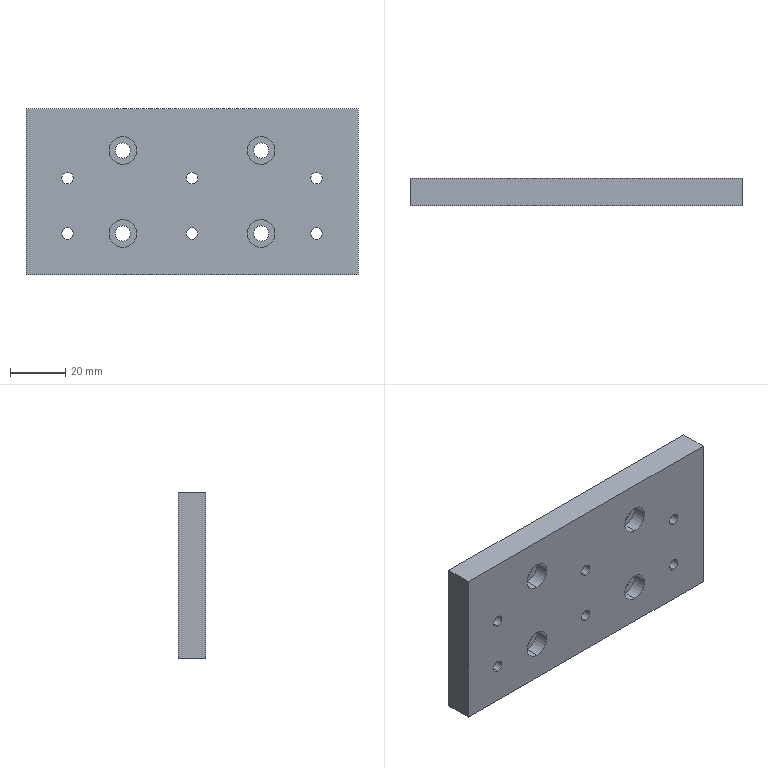Part | SolidWorks | features HoleWzd 2, LPattern 2, Extrusion 1 | 1 solid | 38 faces | box 120 x 10 x 60 mm | volume 69123 mm3 | cylinder 28 | plane 10 | commonest cylinder face diameters 4.2 x12 5.5 x8 10 x8
STEP:
#1=CARTESIAN_POINT('',(45.,10.,-12.9));
#2=VERTEX_POINT('',#1);
#3=CARTESIAN_POINT('',(45.,10.,-17.1));
#4=VERTEX_POINT('',#3);
#5=CARTESIAN_POINT('',(45.,10.,-15.));
#6=DIRECTION('',(0.,-1.,0.));
#7=DIRECTION('',(0.,0.,-1.));
#8=AXIS2_PLACEMENT_3D('',#5,#6,#7);
#9=CIRCLE('',#8,2.1);
#10=EDGE_CURVE('',#2,#4,#9,.T.);
#11=ORIENTED_EDGE('',*,*,#10,.F.);
#12=CARTESIAN_POINT('',(45.,0.,-12.9));
#13=VERTEX_POINT('',#12);
#14=CARTESIAN_POINT('',(45.,0.,-12.9));
#15=DIRECTION('',(0.,-1.,0.));
#16=VECTOR('',#15,1000.);
#17=LINE('',#14,#16);
#18=EDGE_CURVE('',#2,#13,#17,.T.);
#19=ORIENTED_EDGE('',*,*,#18,.T.);
#20=CARTESIAN_POINT('',(45.,0.,-17.1));
#21=VERTEX_POINT('',#20);
#22=CARTESIAN_POINT('',(45.,0.,-15.));
#23=DIRECTION('',(0.,-1.,0.));
#24=DIRECTION('',(0.,0.,-1.));
#25=AXIS2_PLACEMENT_3D('',#22,#23,#24);
#26=CIRCLE('',#25,2.1);
#27=EDGE_CURVE('',#13,#21,#26,.T.);
#28=ORIENTED_EDGE('',*,*,#27,.T.);
#29=CARTESIAN_POINT('',(45.,0.,-17.1));
#30=DIRECTION('',(0.,-1.,0.));
#31=VECTOR('',#30,1000.);
#32=LINE('',#29,#31);
#33=EDGE_CURVE('',#4,#21,#32,.T.);
#34=ORIENTED_EDGE('',*,*,#33,.F.);
#35=EDGE_LOOP('',(#11,#19,#28,#34));
#36=FACE_OUTER_BOUND('',#35,.T.);
#37=CARTESIAN_POINT('',(45.,0.,-15.));
#38=DIRECTION('',(0.,-1.,0.));
#39=DIRECTION('',(0.,0.,-1.));
#40=AXIS2_PLACEMENT_3D('',#37,#38,#39);
#41=CYLINDRICAL_SURFACE('',#40,2.1);
#42=ADVANCED_FACE('',(#36),#41,.F.);
#43=CARTESIAN_POINT('',(0.,10.,-12.9));
#44=VERTEX_POINT('',#43);
#45=CARTESIAN_POINT('',(0.,10.,-17.1));
#46=VERTEX_POINT('',#45);
#47=CARTESIAN_POINT('',(0.,10.,-15.));
#48=DIRECTION('',(0.,-1.,0.));
#49=DIRECTION('',(0.,0.,-1.));
#50=AXIS2_PLACEMENT_3D('',#47,#48,#49);
#51=CIRCLE('',#50,2.1);
#52=EDGE_CURVE('',#44,#46,#51,.T.);
#53=ORIENTED_EDGE('',*,*,#52,.F.);
#54=CARTESIAN_POINT('',(0.,0.,-12.9));
#55=VERTEX_POINT('',#54);
#56=CARTESIAN_POINT('',(0.,0.,-12.9));
#57=DIRECTION('',(0.,-1.,0.));
#58=VECTOR('',#57,1000.);
#59=LINE('',#56,#58);
#60=EDGE_CURVE('',#44,#55,#59,.T.);
#61=ORIENTED_EDGE('',*,*,#60,.T.);
#62=CARTESIAN_POINT('',(0.,0.,-17.1));
#63=VERTEX_POINT('',#62);
#64=CARTESIAN_POINT('',(0.,0.,-15.));
#65=DIRECTION('',(0.,-1.,0.));
#66=DIRECTION('',(0.,0.,-1.));
#67=AXIS2_PLACEMENT_3D('',#64,#65,#66);
#68=CIRCLE('',#67,2.1);
#69=EDGE_CURVE('',#55,#63,#68,.T.);
#70=ORIENTED_EDGE('',*,*,#69,.T.);
#71=CARTESIAN_POINT('',(0.,0.,-17.1));
#72=DIRECTION('',(0.,-1.,0.));
#73=VECTOR('',#72,1000.);
#74=LINE('',#71,#73);
#75=EDGE_CURVE('',#46,#63,#74,.T.);
#76=ORIENTED_EDGE('',*,*,#75,.F.);
#77=EDGE_LOOP('',(#53,#61,#70,#76));
#78=FACE_OUTER_BOUND('',#77,.T.);
#79=CARTESIAN_POINT('',(0.,0.,-15.));
#80=DIRECTION('',(0.,-1.,0.));
#81=DIRECTION('',(0.,0.,-1.));
#82=AXIS2_PLACEMENT_3D('',#79,#80,#81);
#83=CYLINDRICAL_SURFACE('',#82,2.1);
#84=ADVANCED_FACE('',(#78),#83,.F.);
#85=CARTESIAN_POINT('',(-45.,10.,-12.9));
#86=VERTEX_POINT('',#85);
#87=CARTESIAN_POINT('',(-45.,10.,-17.1));
#88=VERTEX_POINT('',#87);
#89=CARTESIAN_POINT('',(-45.,10.,-15.));
#90=DIRECTION('',(0.,-1.,0.));
#91=DIRECTION('',(0.,0.,-1.));
#92=AXIS2_PLACEMENT_3D('',#89,#90,#91);
#93=CIRCLE('',#92,2.1);
#94=EDGE_CURVE('',#86,#88,#93,.T.);
#95=ORIENTED_EDGE('',*,*,#94,.F.);
#96=CARTESIAN_POINT('',(-45.,0.,-12.9));
#97=VERTEX_POINT('',#96);
#98=CARTESIAN_POINT('',(-45.,0.,-12.9));
#99=DIRECTION('',(0.,-1.,0.));
#100=VECTOR('',#99,1000.);
#101=LINE('',#98,#100);
#102=EDGE_CURVE('',#86,#97,#101,.T.);
#103=ORIENTED_EDGE('',*,*,#102,.T.);
#104=CARTESIAN_POINT('',(-45.,0.,-17.1));
#105=VERTEX_POINT('',#104);
#106=CARTESIAN_POINT('',(-45.,0.,-15.));
#107=DIRECTION('',(0.,-1.,0.));
#108=DIRECTION('',(0.,0.,-1.));
#109=AXIS2_PLACEMENT_3D('',#106,#107,#108);
#110=CIRCLE('',#109,2.1);
#111=EDGE_CURVE('',#97,#105,#110,.T.);
#112=ORIENTED_EDGE('',*,*,#111,.T.);
#113=CARTESIAN_POINT('',(-45.,0.,-17.1));
#114=DIRECTION('',(0.,-1.,0.));
#115=VECTOR('',#114,1000.);
#116=LINE('',#113,#115);
#117=EDGE_CURVE('',#88,#105,#116,.T.);
#118=ORIENTED_EDGE('',*,*,#117,.F.);
#119=EDGE_LOOP('',(#95,#103,#112,#118));
#120=FACE_OUTER_BOUND('',#119,.T.);
#121=CARTESIAN_POINT('',(-45.,0.,-15.));
#122=DIRECTION('',(0.,-1.,0.));
#123=DIRECTION('',(0.,0.,-1.));
#124=AXIS2_PLACEMENT_3D('',#121,#122,#123);
#125=CYLINDRICAL_SURFACE('',#124,2.1);
#126=ADVANCED_FACE('',(#120),#125,.F.);
#127=CARTESIAN_POINT('',(45.,10.,7.1));
#128=VERTEX_POINT('',#127);
#129=CARTESIAN_POINT('',(45.,10.,2.9));
#130=VERTEX_POINT('',#129);
#131=CARTESIAN_POINT('',(45.,10.,5.));
#132=DIRECTION('',(0.,-1.,0.));
#133=DIRECTION('',(0.,0.,-1.));
#134=AXIS2_PLACEMENT_3D('',#131,#132,#133);
#135=CIRCLE('',#134,2.1);
#136=EDGE_CURVE('',#128,#130,#135,.T.);
#137=ORIENTED_EDGE('',*,*,#136,.F.);
#138=CARTESIAN_POINT('',(45.,0.,7.1));
#139=VERTEX_POINT('',#138);
#140=CARTESIAN_POINT('',(45.,0.,7.1));
#141=DIRECTION('',(0.,-1.,0.));
#142=VECTOR('',#141,1000.);
#143=LINE('',#140,#142);
#144=EDGE_CURVE('',#128,#139,#143,.T.);
#145=ORIENTED_EDGE('',*,*,#144,.T.);
#146=CARTESIAN_POINT('',(45.,0.,2.9));
#147=VERTEX_POINT('',#146);
#148=CARTESIAN_POINT('',(45.,0.,5.));
#149=DIRECTION('',(0.,-1.,0.));
#150=DIRECTION('',(0.,0.,-1.));
#151=AXIS2_PLACEMENT_3D('',#148,#149,#150);
#152=CIRCLE('',#151,2.1);
#153=EDGE_CURVE('',#139,#147,#152,.T.);
#154=ORIENTED_EDGE('',*,*,#153,.T.);
#155=CARTESIAN_POINT('',(45.,0.,2.9));
#156=DIRECTION('',(0.,-1.,0.));
#157=VECTOR('',#156,1000.);
#158=LINE('',#155,#157);
#159=EDGE_CURVE('',#130,#147,#158,.T.);
#160=ORIENTED_EDGE('',*,*,#159,.F.);
#161=EDGE_LOOP('',(#137,#145,#154,#160));
#162=FACE_OUTER_BOUND('',#161,.T.);
#163=CARTESIAN_POINT('',(45.,0.,5.));
#164=DIRECTION('',(0.,-1.,0.));
#165=DIRECTION('',(0.,0.,-1.));
#166=AXIS2_PLACEMENT_3D('',#163,#164,#165);
#167=CYLINDRICAL_SURFACE('',#166,2.1);
#168=ADVANCED_FACE('',(#162),#167,.F.);
#169=CARTESIAN_POINT('',(0.,10.,7.1));
#170=VERTEX_POINT('',#169);
#171=CARTESIAN_POINT('',(0.,10.,2.9));
#172=VERTEX_POINT('',#171);
#173=CARTESIAN_POINT('',(0.,10.,5.));
#174=DIRECTION('',(0.,-1.,0.));
#175=DIRECTION('',(0.,0.,-1.));
#176=AXIS2_PLACEMENT_3D('',#173,#174,#175);
#177=CIRCLE('',#176,2.1);
#178=EDGE_CURVE('',#170,#172,#177,.T.);
#179=ORIENTED_EDGE('',*,*,#178,.F.);
#180=CARTESIAN_POINT('',(0.,0.,7.1));
#181=VERTEX_POINT('',#180);
#182=CARTESIAN_POINT('',(0.,0.,7.1));
#183=DIRECTION('',(0.,-1.,0.));
#184=VECTOR('',#183,1000.);
#185=LINE('',#182,#184);
#186=EDGE_CURVE('',#170,#181,#185,.T.);
#187=ORIENTED_EDGE('',*,*,#186,.T.);
#188=CARTESIAN_POINT('',(0.,0.,2.9));
#189=VERTEX_POINT('',#188);
#190=CARTESIAN_POINT('',(0.,0.,5.));
#191=DIRECTION('',(0.,-1.,0.));
#192=DIRECTION('',(0.,0.,-1.));
#193=AXIS2_PLACEMENT_3D('',#190,#191,#192);
#194=CIRCLE('',#193,2.1);
#195=EDGE_CURVE('',#181,#189,#194,.T.);
#196=ORIENTED_EDGE('',*,*,#195,.T.);
#197=CARTESIAN_POINT('',(0.,0.,2.9));
#198=DIRECTION('',(0.,-1.,0.));
#199=VECTOR('',#198,1000.);
#200=LINE('',#197,#199);
#201=EDGE_CURVE('',#172,#189,#200,.T.);
#202=ORIENTED_EDGE('',*,*,#201,.F.);
#203=EDGE_LOOP('',(#179,#187,#196,#202));
#204=FACE_OUTER_BOUND('',#203,.T.);
#205=CARTESIAN_POINT('',(0.,0.,5.));
#206=DIRECTION('',(0.,-1.,0.));
#207=DIRECTION('',(0.,0.,-1.));
#208=AXIS2_PLACEMENT_3D('',#205,#206,#207);
#209=CYLINDRICAL_SURFACE('',#208,2.1);
#210=ADVANCED_FACE('',(#204),#209,.F.);
#211=CARTESIAN_POINT('',(-45.,10.,7.1));
#212=VERTEX_POINT('',#211);
#213=CARTESIAN_POINT('',(-45.,10.,2.9));
#214=VERTEX_POINT('',#213);
#215=CARTESIAN_POINT('',(-45.,10.,5.));
#216=DIRECTION('',(0.,-1.,0.));
#217=DIRECTION('',(0.,0.,-1.));
#218=AXIS2_PLACEMENT_3D('',#215,#216,#217);
#219=CIRCLE('',#218,2.1);
#220=EDGE_CURVE('',#212,#214,#219,.T.);
#221=ORIENTED_EDGE('',*,*,#220,.F.);
#222=CARTESIAN_POINT('',(-45.,0.,7.1));
#223=VERTEX_POINT('',#222);
#224=CARTESIAN_POINT('',(-45.,0.,7.1));
#225=DIRECTION('',(0.,-1.,0.));
#226=VECTOR('',#225,1000.);
#227=LINE('',#224,#226);
#228=EDGE_CURVE('',#212,#223,#227,.T.);
#229=ORIENTED_EDGE('',*,*,#228,.T.);
#230=CARTESIAN_POINT('',(-45.,0.,2.9));
#231=VERTEX_POINT('',#230);
#232=CARTESIAN_POINT('',(-45.,0.,5.));
#233=DIRECTION('',(0.,-1.,0.));
#234=DIRECTION('',(0.,0.,-1.));
#235=AXIS2_PLACEMENT_3D('',#232,#233,#234);
#236=CIRCLE('',#235,2.1);
#237=EDGE_CURVE('',#223,#231,#236,.T.);
#238=ORIENTED_EDGE('',*,*,#237,.T.);
#239=CARTESIAN_POINT('',(-45.,0.,2.9));
#240=DIRECTION('',(0.,-1.,0.));
#241=VECTOR('',#240,1000.);
#242=LINE('',#239,#241);
#243=EDGE_CURVE('',#214,#231,#242,.T.);
#244=ORIENTED_EDGE('',*,*,#243,.F.);
#245=EDGE_LOOP('',(#221,#229,#238,#244));
#246=FACE_OUTER_BOUND('',#245,.T.);
#247=CARTESIAN_POINT('',(-45.,0.,5.));
#248=DIRECTION('',(0.,-1.,0.));
#249=DIRECTION('',(0.,0.,-1.));
#250=AXIS2_PLACEMENT_3D('',#247,#248,#249);
#251=CYLINDRICAL_SURFACE('',#250,2.1);
#252=ADVANCED_FACE('',(#246),#251,.F.);
#253=CARTESIAN_POINT('',(25.,10.,-12.25));
#254=VERTEX_POINT('',#253);
#255=CARTESIAN_POINT('',(25.,10.,-17.75));
#256=VERTEX_POINT('',#255);
#257=CARTESIAN_POINT('',(25.,10.,-15.));
#258=DIRECTION('',(0.,-1.,0.));
#259=DIRECTION('',(0.,0.,-1.));
#260=AXIS2_PLACEMENT_3D('',#257,#258,#259);
#261=CIRCLE('',#260,2.75);
#262=EDGE_CURVE('',#254,#256,#261,.T.);
#263=ORIENTED_EDGE('',*,*,#262,.F.);
#264=CARTESIAN_POINT('',(25.,5.,-12.25));
#265=VERTEX_POINT('',#264);
#266=CARTESIAN_POINT('',(25.,0.,-12.25));
#267=DIRECTION('',(0.,-1.,0.));
#268=VECTOR('',#267,1000.);
#269=LINE('',#266,#268);
#270=EDGE_CURVE('',#254,#265,#269,.T.);
#271=ORIENTED_EDGE('',*,*,#270,.T.);
#272=CARTESIAN_POINT('',(25.,5.,-17.75));
#273=VERTEX_POINT('',#272);
#274=CARTESIAN_POINT('',(25.,5.,-15.));
#275=DIRECTION('',(0.,-1.,0.));
#276=DIRECTION('',(0.,0.,-1.));
#277=AXIS2_PLACEMENT_3D('',#274,#275,#276);
#278=CIRCLE('',#277,2.75);
#279=EDGE_CURVE('',#265,#273,#278,.T.);
#280=ORIENTED_EDGE('',*,*,#279,.T.);
#281=CARTESIAN_POINT('',(25.,0.,-17.75));
#282=DIRECTION('',(0.,-1.,0.));
#283=VECTOR('',#282,1000.);
#284=LINE('',#281,#283);
#285=EDGE_CURVE('',#256,#273,#284,.T.);
#286=ORIENTED_EDGE('',*,*,#285,.F.);
#287=EDGE_LOOP('',(#263,#271,#280,#286));
#288=FACE_OUTER_BOUND('',#287,.T.);
#289=CARTESIAN_POINT('',(25.,0.,-15.));
#290=DIRECTION('',(0.,-1.,0.));
#291=DIRECTION('',(0.,0.,-1.));
#292=AXIS2_PLACEMENT_3D('',#289,#290,#291);
#293=CYLINDRICAL_SURFACE('',#292,2.75);
#294=ADVANCED_FACE('',(#288),#293,.F.);
#295=CARTESIAN_POINT('',(25.,5.,-10.));
#296=VERTEX_POINT('',#295);
#297=CARTESIAN_POINT('',(25.,5.,-20.));
#298=VERTEX_POINT('',#297);
#299=CARTESIAN_POINT('',(25.,5.,-15.));
#300=DIRECTION('',(0.,-1.,0.));
#301=DIRECTION('',(0.,0.,-1.));
#302=AXIS2_PLACEMENT_3D('',#299,#300,#301);
#303=CIRCLE('',#302,5.);
#304=EDGE_CURVE('',#296,#298,#303,.T.);
#305=ORIENTED_EDGE('',*,*,#304,.F.);
#306=CARTESIAN_POINT('',(25.,0.,-10.));
#307=VERTEX_POINT('',#306);
#308=CARTESIAN_POINT('',(25.,0.,-10.));
#309=DIRECTION('',(0.,-1.,0.));
#310=VECTOR('',#309,1000.);
#311=LINE('',#308,#310);
#312=EDGE_CURVE('',#296,#307,#311,.T.);
#313=ORIENTED_EDGE('',*,*,#312,.T.);
#314=CARTESIAN_POINT('',(25.,0.,-20.));
#315=VERTEX_POINT('',#314);
#316=CARTESIAN_POINT('',(25.,0.,-15.));
#317=DIRECTION('',(0.,-1.,0.));
#318=DIRECTION('',(0.,0.,-1.));
#319=AXIS2_PLACEMENT_3D('',#316,#317,#318);
#320=CIRCLE('',#319,5.);
#321=EDGE_CURVE('',#307,#315,#320,.T.);
#322=ORIENTED_EDGE('',*,*,#321,.T.);
#323=CARTESIAN_POINT('',(25.,0.,-20.));
#324=DIRECTION('',(0.,-1.,0.));
#325=VECTOR('',#324,1000.);
#326=LINE('',#323,#325);
#327=EDGE_CURVE('',#298,#315,#326,.T.);
#328=ORIENTED_EDGE('',*,*,#327,.F.);
#329=EDGE_LOOP('',(#305,#313,#322,#328));
#330=FACE_OUTER_BOUND('',#329,.T.);
#331=CARTESIAN_POINT('',(25.,0.,-15.));
#332=DIRECTION('',(0.,-1.,0.));
#333=DIRECTION('',(0.,0.,-1.));
#334=AXIS2_PLACEMENT_3D('',#331,#332,#333);
#335=CYLINDRICAL_SURFACE('',#334,5.);
#336=ADVANCED_FACE('',(#330),#335,.F.);
#337=CARTESIAN_POINT('',(-25.,10.,-12.25));
#338=VERTEX_POINT('',#337);
#339=CARTESIAN_POINT('',(-25.,10.,-17.75));
#340=VERTEX_POINT('',#339);
#341=CARTESIAN_POINT('',(-25.,10.,-15.));
#342=DIRECTION('',(0.,-1.,0.));
#343=DIRECTION('',(0.,0.,-1.));
#344=AXIS2_PLACEMENT_3D('',#341,#342,#343);
#345=CIRCLE('',#344,2.75);
#346=EDGE_CURVE('',#338,#340,#345,.T.);
#347=ORIENTED_EDGE('',*,*,#346,.F.);
#348=CARTESIAN_POINT('',(-25.,5.,-12.25));
#349=VERTEX_POINT('',#348);
#350=CARTESIAN_POINT('',(-25.,0.,-12.25));
#351=DIRECTION('',(0.,-1.,0.));
#352=VECTOR('',#351,1000.);
#353=LINE('',#350,#352);
#354=EDGE_CURVE('',#338,#349,#353,.T.);
#355=ORIENTED_EDGE('',*,*,#354,.T.);
#356=CARTESIAN_POINT('',(-25.,5.,-17.75));
#357=VERTEX_POINT('',#356);
#358=CARTESIAN_POINT('',(-25.,5.,-15.));
#359=DIRECTION('',(0.,-1.,0.));
#360=DIRECTION('',(0.,0.,-1.));
#361=AXIS2_PLACEMENT_3D('',#358,#359,#360);
#362=CIRCLE('',#361,2.75);
#363=EDGE_CURVE('',#349,#357,#362,.T.);
#364=ORIENTED_EDGE('',*,*,#363,.T.);
#365=CARTESIAN_POINT('',(-25.,0.,-17.75));
#366=DIRECTION('',(0.,-1.,0.));
#367=VECTOR('',#366,1000.);
#368=LINE('',#365,#367);
#369=EDGE_CURVE('',#340,#357,#368,.T.);
#370=ORIENTED_EDGE('',*,*,#369,.F.);
#371=EDGE_LOOP('',(#347,#355,#364,#370));
#372=FACE_OUTER_BOUND('',#371,.T.);
#373=CARTESIAN_POINT('',(-25.,0.,-15.));
#374=DIRECTION('',(0.,-1.,0.));
#375=DIRECTION('',(0.,0.,-1.));
#376=AXIS2_PLACEMENT_3D('',#373,#374,#375);
#377=CYLINDRICAL_SURFACE('',#376,2.75);
#378=ADVANCED_FACE('',(#372),#377,.F.);
#379=CARTESIAN_POINT('',(-25.,5.,-10.));
#380=VERTEX_POINT('',#379);
#381=CARTESIAN_POINT('',(-25.,5.,-20.));
#382=VERTEX_POINT('',#381);
#383=CARTESIAN_POINT('',(-25.,5.,-15.));
#384=DIRECTION('',(0.,-1.,0.));
#385=DIRECTION('',(0.,0.,-1.));
#386=AXIS2_PLACEMENT_3D('',#383,#384,#385);
#387=CIRCLE('',#386,5.);
#388=EDGE_CURVE('',#380,#382,#387,.T.);
#389=ORIENTED_EDGE('',*,*,#388,.F.);
#390=CARTESIAN_POINT('',(-25.,0.,-10.));
#391=VERTEX_POINT('',#390);
#392=CARTESIAN_POINT('',(-25.,0.,-10.));
#393=DIRECTION('',(0.,-1.,0.));
#394=VECTOR('',#393,1000.);
#395=LINE('',#392,#394);
#396=EDGE_CURVE('',#380,#391,#395,.T.);
#397=ORIENTED_EDGE('',*,*,#396,.T.);
#398=CARTESIAN_POINT('',(-25.,0.,-20.));
#399=VERTEX_POINT('',#398);
#400=CARTESIAN_POINT('',(-25.,0.,-15.));
#401=DIRECTION('',(0.,-1.,0.));
#402=DIRECTION('',(0.,0.,-1.));
#403=AXIS2_PLACEMENT_3D('',#400,#401,#402);
#404=CIRCLE('',#403,5.);
#405=EDGE_CURVE('',#391,#399,#404,.T.);
#406=ORIENTED_EDGE('',*,*,#405,.T.);
#407=CARTESIAN_POINT('',(-25.,0.,-20.));
#408=DIRECTION('',(0.,-1.,0.));
#409=VECTOR('',#408,1000.);
#410=LINE('',#407,#409);
#411=EDGE_CURVE('',#382,#399,#410,.T.);
#412=ORIENTED_EDGE('',*,*,#411,.F.);
#413=EDGE_LOOP('',(#389,#397,#406,#412));
#414=FACE_OUTER_BOUND('',#413,.T.);
#415=CARTESIAN_POINT('',(-25.,0.,-15.));
#416=DIRECTION('',(0.,-1.,0.));
#417=DIRECTION('',(0.,0.,-1.));
#418=AXIS2_PLACEMENT_3D('',#415,#416,#417);
#419=CYLINDRICAL_SURFACE('',#418,5.);
#420=ADVANCED_FACE('',(#414),#419,.F.);
#421=CARTESIAN_POINT('',(25.,5.,20.));
#422=VERTEX_POINT('',#421);
#423=CARTESIAN_POINT('',(25.,5.,10.));
#424=VERTEX_POINT('',#423);
#425=CARTESIAN_POINT('',(25.,5.,15.));
#426=DIRECTION('',(0.,-1.,0.));
#427=DIRECTION('',(0.,0.,-1.));
#428=AXIS2_PLACEMENT_3D('',#425,#426,#427);
#429=CIRCLE('',#428,5.);
#430=EDGE_CURVE('',#422,#424,#429,.T.);
#431=ORIENTED_EDGE('',*,*,#430,.F.);
#432=CARTESIAN_POINT('',(25.,0.,20.));
#433=VERTEX_POINT('',#432);
#434=CARTESIAN_POINT('',(25.,0.,20.));
#435=DIRECTION('',(0.,-1.,0.));
#436=VECTOR('',#435,1000.);
#437=LINE('',#434,#436);
#438=EDGE_CURVE('',#422,#433,#437,.T.);
#439=ORIENTED_EDGE('',*,*,#438,.T.);
#440=CARTESIAN_POINT('',(25.,0.,10.));
#441=VERTEX_POINT('',#440);
#442=CARTESIAN_POINT('',(25.,0.,15.));
#443=DIRECTION('',(0.,-1.,0.));
#444=DIRECTION('',(0.,0.,-1.));
#445=AXIS2_PLACEMENT_3D('',#442,#443,#444);
#446=CIRCLE('',#445,5.);
#447=EDGE_CURVE('',#433,#441,#446,.T.);
#448=ORIENTED_EDGE('',*,*,#447,.T.);
#449=CARTESIAN_POINT('',(25.,0.,10.));
#450=DIRECTION('',(0.,-1.,0.));
#451=VECTOR('',#450,1000.);
#452=LINE('',#449,#451);
#453=EDGE_CURVE('',#424,#441,#452,.T.);
#454=ORIENTED_EDGE('',*,*,#453,.F.);
#455=EDGE_LOOP('',(#431,#439,#448,#454));
#456=FACE_OUTER_BOUND('',#455,.T.);
#457=CARTESIAN_POINT('',(25.,0.,15.));
#458=DIRECTION('',(0.,-1.,0.));
#459=DIRECTION('',(0.,0.,-1.));
#460=AXIS2_PLACEMENT_3D('',#457,#458,#459);
#461=CYLINDRICAL_SURFACE('',#460,5.);
#462=ADVANCED_FACE('',(#456),#461,.F.);
#463=CARTESIAN_POINT('',(25.,10.,17.75));
#464=VERTEX_POINT('',#463);
#465=CARTESIAN_POINT('',(25.,10.,12.25));
#466=VERTEX_POINT('',#465);
#467=CARTESIAN_POINT('',(25.,10.,15.));
#468=DIRECTION('',(0.,-1.,0.));
#469=DIRECTION('',(0.,0.,-1.));
#470=AXIS2_PLACEMENT_3D('',#467,#468,#469);
#471=CIRCLE('',#470,2.75);
#472=EDGE_CURVE('',#464,#466,#471,.T.);
#473=ORIENTED_EDGE('',*,*,#472,.F.);
#474=CARTESIAN_POINT('',(25.,5.,17.75));
#475=VERTEX_POINT('',#474);
#476=CARTESIAN_POINT('',(25.,0.,17.75));
#477=DIRECTION('',(0.,-1.,0.));
#478=VECTOR('',#477,1000.);
#479=LINE('',#476,#478);
#480=EDGE_CURVE('',#464,#475,#479,.T.);
#481=ORIENTED_EDGE('',*,*,#480,.T.);
#482=CARTESIAN_POINT('',(25.,5.,12.25));
#483=VERTEX_POINT('',#482);
#484=CARTESIAN_POINT('',(25.,5.,15.));
#485=DIRECTION('',(0.,-1.,0.));
#486=DIRECTION('',(0.,0.,-1.));
#487=AXIS2_PLACEMENT_3D('',#484,#485,#486);
#488=CIRCLE('',#487,2.75);
#489=EDGE_CURVE('',#475,#483,#488,.T.);
#490=ORIENTED_EDGE('',*,*,#489,.T.);
#491=CARTESIAN_POINT('',(25.,0.,12.25));
#492=DIRECTION('',(0.,-1.,0.));
#493=VECTOR('',#492,1000.);
#494=LINE('',#491,#493);
#495=EDGE_CURVE('',#466,#483,#494,.T.);
#496=ORIENTED_EDGE('',*,*,#495,.F.);
#497=EDGE_LOOP('',(#473,#481,#490,#496));
#498=FACE_OUTER_BOUND('',#497,.T.);
#499=CARTESIAN_POINT('',(25.,0.,15.));
#500=DIRECTION('',(0.,-1.,0.));
#501=DIRECTION('',(0.,0.,-1.));
#502=AXIS2_PLACEMENT_3D('',#499,#500,#501);
#503=CYLINDRICAL_SURFACE('',#502,2.75);
#504=ADVANCED_FACE('',(#498),#503,.F.);
#505=CARTESIAN_POINT('',(-25.,5.,20.));
#506=VERTEX_POINT('',#505);
#507=CARTESIAN_POINT('',(-25.,5.,10.));
#508=VERTEX_POINT('',#507);
#509=CARTESIAN_POINT('',(-25.,5.,15.));
#510=DIRECTION('',(0.,-1.,0.));
#511=DIRECTION('',(0.,0.,-1.));
#512=AXIS2_PLACEMENT_3D('',#509,#510,#511);
#513=CIRCLE('',#512,5.);
#514=EDGE_CURVE('',#506,#508,#513,.T.);
#515=ORIENTED_EDGE('',*,*,#514,.F.);
#516=CARTESIAN_POINT('',(-25.,0.,20.));
#517=VERTEX_POINT('',#516);
#518=CARTESIAN_POINT('',(-25.,0.,20.));
#519=DIRECTION('',(0.,-1.,0.));
#520=VECTOR('',#519,1000.);
#521=LINE('',#518,#520);
#522=EDGE_CURVE('',#506,#517,#521,.T.);
#523=ORIENTED_EDGE('',*,*,#522,.T.);
#524=CARTESIAN_POINT('',(-25.,0.,10.));
#525=VERTEX_POINT('',#524);
#526=CARTESIAN_POINT('',(-25.,0.,15.));
#527=DIRECTION('',(0.,-1.,0.));
#528=DIRECTION('',(0.,0.,-1.));
#529=AXIS2_PLACEMENT_3D('',#526,#527,#528);
#530=CIRCLE('',#529,5.);
#531=EDGE_CURVE('',#517,#525,#530,.T.);
#532=ORIENTED_EDGE('',*,*,#531,.T.);
#533=CARTESIAN_POINT('',(-25.,0.,10.));
#534=DIRECTION('',(0.,-1.,0.));
#535=VECTOR('',#534,1000.);
#536=LINE('',#533,#535);
#537=EDGE_CURVE('',#508,#525,#536,.T.);
#538=ORIENTED_EDGE('',*,*,#537,.F.);
#539=EDGE_LOOP('',(#515,#523,#532,#538));
#540=FACE_OUTER_BOUND('',#539,.T.);
#541=CARTESIAN_POINT('',(-25.,0.,15.));
#542=DIRECTION('',(0.,-1.,0.));
#543=DIRECTION('',(0.,0.,-1.));
#544=AXIS2_PLACEMENT_3D('',#541,#542,#543);
#545=CYLINDRICAL_SURFACE('',#544,5.);
#546=ADVANCED_FACE('',(#540),#545,.F.);
#547=CARTESIAN_POINT('',(-25.,10.,17.75));
#548=VERTEX_POINT('',#547);
#549=CARTESIAN_POINT('',(-25.,10.,12.25));
#550=VERTEX_POINT('',#549);
#551=CARTESIAN_POINT('',(-25.,10.,15.));
#552=DIRECTION('',(0.,-1.,0.));
#553=DIRECTION('',(0.,0.,-1.));
#554=AXIS2_PLACEMENT_3D('',#551,#552,#553);
#555=CIRCLE('',#554,2.75);
#556=EDGE_CURVE('',#548,#550,#555,.T.);
#557=ORIENTED_EDGE('',*,*,#556,.F.);
#558=CARTESIAN_POINT('',(-25.,5.,17.75));
#559=VERTEX_POINT('',#558);
#560=CARTESIAN_POINT('',(-25.,0.,17.75));
#561=DIRECTION('',(0.,-1.,0.));
#562=VECTOR('',#561,1000.);
#563=LINE('',#560,#562);
#564=EDGE_CURVE('',#548,#559,#563,.T.);
#565=ORIENTED_EDGE('',*,*,#564,.T.);
#566=CARTESIAN_POINT('',(-25.,5.,12.25));
#567=VERTEX_POINT('',#566);
#568=CARTESIAN_POINT('',(-25.,5.,15.));
#569=DIRECTION('',(0.,-1.,0.));
#570=DIRECTION('',(0.,0.,-1.));
#571=AXIS2_PLACEMENT_3D('',#568,#569,#570);
#572=CIRCLE('',#571,2.75);
#573=EDGE_CURVE('',#559,#567,#572,.T.);
#574=ORIENTED_EDGE('',*,*,#573,.T.);
#575=CARTESIAN_POINT('',(-25.,0.,12.25));
#576=DIRECTION('',(0.,-1.,0.));
#577=VECTOR('',#576,1000.);
#578=LINE('',#575,#577);
#579=EDGE_CURVE('',#550,#567,#578,.T.);
#580=ORIENTED_EDGE('',*,*,#579,.F.);
#581=EDGE_LOOP('',(#557,#565,#574,#580));
#582=FACE_OUTER_BOUND('',#581,.T.);
#583=CARTESIAN_POINT('',(-25.,0.,15.));
#584=DIRECTION('',(0.,-1.,0.));
#585=DIRECTION('',(0.,0.,-1.));
#586=AXIS2_PLACEMENT_3D('',#583,#584,#585);
#587=CYLINDRICAL_SURFACE('',#586,2.75);
#588=ADVANCED_FACE('',(#582),#587,.F.);
#589=CARTESIAN_POINT('',(60.,0.,30.));
#590=VERTEX_POINT('',#589);
#591=CARTESIAN_POINT('',(60.,0.,-30.));
#592=VERTEX_POINT('',#591);
#593=CARTESIAN_POINT('',(60.,0.,30.));
#594=DIRECTION('',(0.,0.,-1.));
#595=VECTOR('',#594,1000.);
#596=LINE('',#593,#595);
#597=EDGE_CURVE('',#590,#592,#596,.T.);
#598=ORIENTED_EDGE('',*,*,#597,.T.);
#599=CARTESIAN_POINT('',(60.,10.,-30.));
#600=VERTEX_POINT('',#599);
#601=CARTESIAN_POINT('',(60.,10.,-30.));
#602=DIRECTION('',(0.,-1.,0.));
#603=VECTOR('',#602,1000.);
#604=LINE('',#601,#603);
#605=EDGE_CURVE('',#600,#592,#604,.T.);
#606=ORIENTED_EDGE('',*,*,#605,.F.);
#607=CARTESIAN_POINT('',(60.,10.,30.));
#608=VERTEX_POINT('',#607);
#609=CARTESIAN_POINT('',(60.,10.,30.));
#610=DIRECTION('',(0.,0.,-1.));
#611=VECTOR('',#610,1000.);
#612=LINE('',#609,#611);
#613=EDGE_CURVE('',#608,#600,#612,.T.);
#614=ORIENTED_EDGE('',*,*,#613,.F.);
#615=CARTESIAN_POINT('',(60.,10.,30.));
#616=DIRECTION('',(0.,-1.,0.));
#617=VECTOR('',#616,1000.);
#618=LINE('',#615,#617);
#619=EDGE_CURVE('',#608,#590,#618,.T.);
#620=ORIENTED_EDGE('',*,*,#619,.T.);
#621=EDGE_LOOP('',(#598,#606,#614,#620));
#622=FACE_OUTER_BOUND('',#621,.T.);
#623=CARTESIAN_POINT('',(60.,10.,30.));
#624=DIRECTION('',(-1.,0.,0.));
#625=DIRECTION('',(0.,0.,1.));
#626=AXIS2_PLACEMENT_3D('',#623,#624,#625);
#627=PLANE('',#626);
#628=ADVANCED_FACE('',(#622),#627,.F.);
#629=CARTESIAN_POINT('',(-60.,0.,-30.));
#630=VERTEX_POINT('',#629);
#631=CARTESIAN_POINT('',(-60.,0.,-30.));
#632=DIRECTION('',(-1.,0.,0.));
#633=VECTOR('',#632,1000.);
#634=LINE('',#631,#633);
#635=EDGE_CURVE('',#592,#630,#634,.T.);
#636=ORIENTED_EDGE('',*,*,#635,.T.);
#637=CARTESIAN_POINT('',(-60.,10.,-30.));
#638=VERTEX_POINT('',#637);
#639=CARTESIAN_POINT('',(-60.,10.,-30.));
#640=DIRECTION('',(0.,-1.,0.));
#641=VECTOR('',#640,1000.);
#642=LINE('',#639,#641);
#643=EDGE_CURVE('',#638,#630,#642,.T.);
#644=ORIENTED_EDGE('',*,*,#643,.F.);
#645=CARTESIAN_POINT('',(-60.,10.,-30.));
#646=DIRECTION('',(-1.,0.,0.));
#647=VECTOR('',#646,1000.);
#648=LINE('',#645,#647);
#649=EDGE_CURVE('',#600,#638,#648,.T.);
#650=ORIENTED_EDGE('',*,*,#649,.F.);
#651=ORIENTED_EDGE('',*,*,#605,.T.);
#652=EDGE_LOOP('',(#636,#644,#650,#651));
#653=FACE_OUTER_BOUND('',#652,.T.);
#654=CARTESIAN_POINT('',(-60.,10.,-30.));
#655=DIRECTION('',(0.,0.,1.));
#656=DIRECTION('',(1.,0.,0.));
#657=AXIS2_PLACEMENT_3D('',#654,#655,#656);
#658=PLANE('',#657);
#659=ADVANCED_FACE('',(#653),#658,.F.);
#660=CARTESIAN_POINT('',(-60.,0.,30.));
#661=VERTEX_POINT('',#660);
#662=CARTESIAN_POINT('',(-60.,0.,30.));
#663=DIRECTION('',(0.,0.,1.));
#664=VECTOR('',#663,1000.);
#665=LINE('',#662,#664);
#666=EDGE_CURVE('',#630,#661,#665,.T.);
#667=ORIENTED_EDGE('',*,*,#666,.T.);
#668=CARTESIAN_POINT('',(-60.,10.,30.));
#669=VERTEX_POINT('',#668);
#670=CARTESIAN_POINT('',(-60.,10.,30.));
#671=DIRECTION('',(0.,-1.,0.));
#672=VECTOR('',#671,1000.);
#673=LINE('',#670,#672);
#674=EDGE_CURVE('',#669,#661,#673,.T.);
#675=ORIENTED_EDGE('',*,*,#674,.F.);
#676=CARTESIAN_POINT('',(-60.,10.,30.));
#677=DIRECTION('',(0.,0.,1.));
#678=VECTOR('',#677,1000.);
#679=LINE('',#676,#678);
#680=EDGE_CURVE('',#638,#669,#679,.T.);
#681=ORIENTED_EDGE('',*,*,#680,.F.);
#682=ORIENTED_EDGE('',*,*,#643,.T.);
#683=EDGE_LOOP('',(#667,#675,#681,#682));
#684=FACE_OUTER_BOUND('',#683,.T.);
#685=CARTESIAN_POINT('',(-60.,10.,30.));
#686=DIRECTION('',(1.,0.,0.));
#687=DIRECTION('',(0.,0.,-1.));
#688=AXIS2_PLACEMENT_3D('',#685,#686,#687);
#689=PLANE('',#688);
#690=ADVANCED_FACE('',(#684),#689,.F.);
#691=CARTESIAN_POINT('',(-60.,0.,30.));
#692=DIRECTION('',(1.,0.,0.));
#693=VECTOR('',#692,1000.);
#694=LINE('',#691,#693);
#695=EDGE_CURVE('',#661,#590,#694,.T.);
#696=ORIENTED_EDGE('',*,*,#695,.T.);
#697=ORIENTED_EDGE('',*,*,#619,.F.);
#698=CARTESIAN_POINT('',(-60.,10.,30.));
#699=DIRECTION('',(1.,0.,0.));
#700=VECTOR('',#699,1000.);
#701=LINE('',#698,#700);
#702=EDGE_CURVE('',#669,#608,#701,.T.);
#703=ORIENTED_EDGE('',*,*,#702,.F.);
#704=ORIENTED_EDGE('',*,*,#674,.T.);
#705=EDGE_LOOP('',(#696,#697,#703,#704));
#706=FACE_OUTER_BOUND('',#705,.T.);
#707=CARTESIAN_POINT('',(-60.,10.,30.));
#708=DIRECTION('',(0.,0.,-1.));
#709=DIRECTION('',(-1.,0.,0.));
#710=AXIS2_PLACEMENT_3D('',#707,#708,#709);
#711=PLANE('',#710);
#712=ADVANCED_FACE('',(#706),#711,.F.);
#713=CARTESIAN_POINT('',(45.,10.,-15.));
#714=DIRECTION('',(0.,-1.,0.));
#715=DIRECTION('',(0.,0.,-1.));
#716=AXIS2_PLACEMENT_3D('',#713,#714,#715);
#717=CIRCLE('',#716,2.1);
#718=EDGE_CURVE('',#4,#2,#717,.T.);
#719=ORIENTED_EDGE('',*,*,#718,.T.);
#720=ORIENTED_EDGE('',*,*,#10,.T.);
#721=EDGE_LOOP('',(#719,#720));
#722=FACE_BOUND('',#721,.T.);
#723=CARTESIAN_POINT('',(0.,10.,-15.));
#724=DIRECTION('',(0.,-1.,0.));
#725=DIRECTION('',(0.,0.,-1.));
#726=AXIS2_PLACEMENT_3D('',#723,#724,#725);
#727=CIRCLE('',#726,2.1);
#728=EDGE_CURVE('',#46,#44,#727,.T.);
#729=ORIENTED_EDGE('',*,*,#728,.T.);
#730=ORIENTED_EDGE('',*,*,#52,.T.);
#731=EDGE_LOOP('',(#729,#730));
#732=FACE_BOUND('',#731,.T.);
#733=CARTESIAN_POINT('',(-45.,10.,-15.));
#734=DIRECTION('',(0.,-1.,0.));
#735=DIRECTION('',(0.,0.,-1.));
#736=AXIS2_PLACEMENT_3D('',#733,#734,#735);
#737=CIRCLE('',#736,2.1);
#738=EDGE_CURVE('',#88,#86,#737,.T.);
#739=ORIENTED_EDGE('',*,*,#738,.T.);
#740=ORIENTED_EDGE('',*,*,#94,.T.);
#741=EDGE_LOOP('',(#739,#740));
#742=FACE_BOUND('',#741,.T.);
#743=CARTESIAN_POINT('',(45.,10.,5.));
#744=DIRECTION('',(0.,-1.,0.));
#745=DIRECTION('',(0.,0.,-1.));
#746=AXIS2_PLACEMENT_3D('',#743,#744,#745);
#747=CIRCLE('',#746,2.1);
#748=EDGE_CURVE('',#130,#128,#747,.T.);
#749=ORIENTED_EDGE('',*,*,#748,.T.);
#750=ORIENTED_EDGE('',*,*,#136,.T.);
#751=EDGE_LOOP('',(#749,#750));
#752=FACE_BOUND('',#751,.T.);
#753=CARTESIAN_POINT('',(0.,10.,5.));
#754=DIRECTION('',(0.,-1.,0.));
#755=DIRECTION('',(0.,0.,-1.));
#756=AXIS2_PLACEMENT_3D('',#753,#754,#755);
#757=CIRCLE('',#756,2.1);
#758=EDGE_CURVE('',#172,#170,#757,.T.);
#759=ORIENTED_EDGE('',*,*,#758,.T.);
#760=ORIENTED_EDGE('',*,*,#178,.T.);
#761=EDGE_LOOP('',(#759,#760));
#762=FACE_BOUND('',#761,.T.);
#763=CARTESIAN_POINT('',(-45.,10.,5.));
#764=DIRECTION('',(0.,-1.,0.));
#765=DIRECTION('',(0.,0.,-1.));
#766=AXIS2_PLACEMENT_3D('',#763,#764,#765);
#767=CIRCLE('',#766,2.1);
#768=EDGE_CURVE('',#214,#212,#767,.T.);
#769=ORIENTED_EDGE('',*,*,#768,.T.);
#770=ORIENTED_EDGE('',*,*,#220,.T.);
#771=EDGE_LOOP('',(#769,#770));
#772=FACE_BOUND('',#771,.T.);
#773=CARTESIAN_POINT('',(25.,10.,15.));
#774=DIRECTION('',(0.,-1.,0.));
#775=DIRECTION('',(0.,0.,-1.));
#776=AXIS2_PLACEMENT_3D('',#773,#774,#775);
#777=CIRCLE('',#776,2.75);
#778=EDGE_CURVE('',#466,#464,#777,.T.);
#779=ORIENTED_EDGE('',*,*,#778,.T.);
#780=ORIENTED_EDGE('',*,*,#472,.T.);
#781=EDGE_LOOP('',(#779,#780));
#782=FACE_BOUND('',#781,.T.);
#783=CARTESIAN_POINT('',(-25.,10.,15.));
#784=DIRECTION('',(0.,-1.,0.));
#785=DIRECTION('',(0.,0.,-1.));
#786=AXIS2_PLACEMENT_3D('',#783,#784,#785);
#787=CIRCLE('',#786,2.75);
#788=EDGE_CURVE('',#550,#548,#787,.T.);
#789=ORIENTED_EDGE('',*,*,#788,.T.);
#790=ORIENTED_EDGE('',*,*,#556,.T.);
#791=EDGE_LOOP('',(#789,#790));
#792=FACE_BOUND('',#791,.T.);
#793=ORIENTED_EDGE('',*,*,#613,.T.);
#794=ORIENTED_EDGE('',*,*,#649,.T.);
#795=ORIENTED_EDGE('',*,*,#680,.T.);
#796=ORIENTED_EDGE('',*,*,#702,.T.);
#797=EDGE_LOOP('',(#793,#794,#795,#796));
#798=FACE_OUTER_BOUND('',#797,.T.);
#799=CARTESIAN_POINT('',(-25.,10.,-15.));
#800=DIRECTION('',(0.,-1.,0.));
#801=DIRECTION('',(0.,0.,-1.));
#802=AXIS2_PLACEMENT_3D('',#799,#800,#801);
#803=CIRCLE('',#802,2.75);
#804=EDGE_CURVE('',#340,#338,#803,.T.);
#805=ORIENTED_EDGE('',*,*,#804,.T.);
#806=ORIENTED_EDGE('',*,*,#346,.T.);
#807=EDGE_LOOP('',(#805,#806));
#808=FACE_BOUND('',#807,.T.);
#809=CARTESIAN_POINT('',(25.,10.,-15.));
#810=DIRECTION('',(0.,-1.,0.));
#811=DIRECTION('',(0.,0.,-1.));
#812=AXIS2_PLACEMENT_3D('',#809,#810,#811);
#813=CIRCLE('',#812,2.75);
#814=EDGE_CURVE('',#256,#254,#813,.T.);
#815=ORIENTED_EDGE('',*,*,#814,.T.);
#816=ORIENTED_EDGE('',*,*,#262,.T.);
#817=EDGE_LOOP('',(#815,#816));
#818=FACE_BOUND('',#817,.T.);
#819=CARTESIAN_POINT('',(60.,10.,-30.));
#820=DIRECTION('',(0.,-1.,0.));
#821=DIRECTION('',(0.,0.,-1.));
#822=AXIS2_PLACEMENT_3D('',#819,#820,#821);
#823=PLANE('',#822);
#824=ADVANCED_FACE('',(#722,#732,#742,#752,#762,#772,#782,#792,#798,#808,#818),#823,.F.);
#825=CARTESIAN_POINT('',(45.,0.,-15.));
#826=DIRECTION('',(0.,-1.,0.));
#827=DIRECTION('',(0.,0.,-1.));
#828=AXIS2_PLACEMENT_3D('',#825,#826,#827);
#829=CIRCLE('',#828,2.1);
#830=EDGE_CURVE('',#21,#13,#829,.T.);
#831=ORIENTED_EDGE('',*,*,#830,.F.);
#832=ORIENTED_EDGE('',*,*,#27,.F.);
#833=EDGE_LOOP('',(#831,#832));
#834=FACE_BOUND('',#833,.T.);
#835=CARTESIAN_POINT('',(0.,0.,-15.));
#836=DIRECTION('',(0.,-1.,0.));
#837=DIRECTION('',(0.,0.,-1.));
#838=AXIS2_PLACEMENT_3D('',#835,#836,#837);
#839=CIRCLE('',#838,2.1);
#840=EDGE_CURVE('',#63,#55,#839,.T.);
#841=ORIENTED_EDGE('',*,*,#840,.F.);
#842=ORIENTED_EDGE('',*,*,#69,.F.);
#843=EDGE_LOOP('',(#841,#842));
#844=FACE_BOUND('',#843,.T.);
#845=CARTESIAN_POINT('',(-45.,0.,-15.));
#846=DIRECTION('',(0.,-1.,0.));
#847=DIRECTION('',(0.,0.,-1.));
#848=AXIS2_PLACEMENT_3D('',#845,#846,#847);
#849=CIRCLE('',#848,2.1);
#850=EDGE_CURVE('',#105,#97,#849,.T.);
#851=ORIENTED_EDGE('',*,*,#850,.F.);
#852=ORIENTED_EDGE('',*,*,#111,.F.);
#853=EDGE_LOOP('',(#851,#852));
#854=FACE_BOUND('',#853,.T.);
#855=CARTESIAN_POINT('',(45.,0.,5.));
#856=DIRECTION('',(0.,-1.,0.));
#857=DIRECTION('',(0.,0.,-1.));
#858=AXIS2_PLACEMENT_3D('',#855,#856,#857);
#859=CIRCLE('',#858,2.1);
#860=EDGE_CURVE('',#147,#139,#859,.T.);
#861=ORIENTED_EDGE('',*,*,#860,.F.);
#862=ORIENTED_EDGE('',*,*,#153,.F.);
#863=EDGE_LOOP('',(#861,#862));
#864=FACE_BOUND('',#863,.T.);
#865=CARTESIAN_POINT('',(0.,0.,5.));
#866=DIRECTION('',(0.,-1.,0.));
#867=DIRECTION('',(0.,0.,-1.));
#868=AXIS2_PLACEMENT_3D('',#865,#866,#867);
#869=CIRCLE('',#868,2.1);
#870=EDGE_CURVE('',#189,#181,#869,.T.);
#871=ORIENTED_EDGE('',*,*,#870,.F.);
#872=ORIENTED_EDGE('',*,*,#195,.F.);
#873=EDGE_LOOP('',(#871,#872));
#874=FACE_BOUND('',#873,.T.);
#875=CARTESIAN_POINT('',(-45.,0.,5.));
#876=DIRECTION('',(0.,-1.,0.));
#877=DIRECTION('',(0.,0.,-1.));
#878=AXIS2_PLACEMENT_3D('',#875,#876,#877);
#879=CIRCLE('',#878,2.1);
#880=EDGE_CURVE('',#231,#223,#879,.T.);
#881=ORIENTED_EDGE('',*,*,#880,.F.);
#882=ORIENTED_EDGE('',*,*,#237,.F.);
#883=EDGE_LOOP('',(#881,#882));
#884=FACE_BOUND('',#883,.T.);
#885=CARTESIAN_POINT('',(25.,0.,15.));
#886=DIRECTION('',(0.,-1.,0.));
#887=DIRECTION('',(0.,0.,-1.));
#888=AXIS2_PLACEMENT_3D('',#885,#886,#887);
#889=CIRCLE('',#888,5.);
#890=EDGE_CURVE('',#441,#433,#889,.T.);
#891=ORIENTED_EDGE('',*,*,#890,.F.);
#892=ORIENTED_EDGE('',*,*,#447,.F.);
#893=EDGE_LOOP('',(#891,#892));
#894=FACE_BOUND('',#893,.T.);
#895=CARTESIAN_POINT('',(-25.,0.,15.));
#896=DIRECTION('',(0.,-1.,0.));
#897=DIRECTION('',(0.,0.,-1.));
#898=AXIS2_PLACEMENT_3D('',#895,#896,#897);
#899=CIRCLE('',#898,5.);
#900=EDGE_CURVE('',#525,#517,#899,.T.);
#901=ORIENTED_EDGE('',*,*,#900,.F.);
#902=ORIENTED_EDGE('',*,*,#531,.F.);
#903=EDGE_LOOP('',(#901,#902));
#904=FACE_BOUND('',#903,.T.);
#905=ORIENTED_EDGE('',*,*,#597,.F.);
#906=ORIENTED_EDGE('',*,*,#695,.F.);
#907=ORIENTED_EDGE('',*,*,#666,.F.);
#908=ORIENTED_EDGE('',*,*,#635,.F.);
#909=EDGE_LOOP('',(#905,#906,#907,#908));
#910=FACE_OUTER_BOUND('',#909,.T.);
#911=CARTESIAN_POINT('',(-25.,0.,-15.));
#912=DIRECTION('',(0.,-1.,0.));
#913=DIRECTION('',(0.,0.,-1.));
#914=AXIS2_PLACEMENT_3D('',#911,#912,#913);
#915=CIRCLE('',#914,5.);
#916=EDGE_CURVE('',#399,#391,#915,.T.);
#917=ORIENTED_EDGE('',*,*,#916,.F.);
#918=ORIENTED_EDGE('',*,*,#405,.F.);
#919=EDGE_LOOP('',(#917,#918));
#920=FACE_BOUND('',#919,.T.);
#921=CARTESIAN_POINT('',(25.,0.,-15.));
#922=DIRECTION('',(0.,-1.,0.));
#923=DIRECTION('',(0.,0.,-1.));
#924=AXIS2_PLACEMENT_3D('',#921,#922,#923);
#925=CIRCLE('',#924,5.);
#926=EDGE_CURVE('',#315,#307,#925,.T.);
#927=ORIENTED_EDGE('',*,*,#926,.F.);
#928=ORIENTED_EDGE('',*,*,#321,.F.);
#929=EDGE_LOOP('',(#927,#928));
#930=FACE_BOUND('',#929,.T.);
#931=CARTESIAN_POINT('',(60.,0.,-30.));
#932=DIRECTION('',(0.,-1.,0.));
#933=DIRECTION('',(0.,0.,-1.));
#934=AXIS2_PLACEMENT_3D('',#931,#932,#933);
#935=PLANE('',#934);
#936=ADVANCED_FACE('',(#834,#844,#854,#864,#874,#884,#894,#904,#910,#920,#930),#935,.T.);
#937=ORIENTED_EDGE('',*,*,#564,.F.);
#938=ORIENTED_EDGE('',*,*,#788,.F.);
#939=ORIENTED_EDGE('',*,*,#579,.T.);
#940=CARTESIAN_POINT('',(-25.,5.,15.));
#941=DIRECTION('',(0.,-1.,0.));
#942=DIRECTION('',(0.,0.,-1.));
#943=AXIS2_PLACEMENT_3D('',#940,#941,#942);
#944=CIRCLE('',#943,2.75);
#945=EDGE_CURVE('',#567,#559,#944,.T.);
#946=ORIENTED_EDGE('',*,*,#945,.T.);
#947=EDGE_LOOP('',(#937,#938,#939,#946));
#948=FACE_OUTER_BOUND('',#947,.T.);
#949=CARTESIAN_POINT('',(-25.,0.,15.));
#950=DIRECTION('',(0.,-1.,0.));
#951=DIRECTION('',(0.,0.,-1.));
#952=AXIS2_PLACEMENT_3D('',#949,#950,#951);
#953=CYLINDRICAL_SURFACE('',#952,2.75);
#954=ADVANCED_FACE('',(#948),#953,.F.);
#955=ORIENTED_EDGE('',*,*,#945,.F.);
#956=ORIENTED_EDGE('',*,*,#573,.F.);
#957=EDGE_LOOP('',(#955,#956));
#958=FACE_BOUND('',#957,.T.);
#959=CARTESIAN_POINT('',(-25.,5.,15.));
#960=DIRECTION('',(0.,-1.,0.));
#961=DIRECTION('',(0.,0.,-1.));
#962=AXIS2_PLACEMENT_3D('',#959,#960,#961);
#963=CIRCLE('',#962,5.);
#964=EDGE_CURVE('',#508,#506,#963,.T.);
#965=ORIENTED_EDGE('',*,*,#964,.T.);
#966=ORIENTED_EDGE('',*,*,#514,.T.);
#967=EDGE_LOOP('',(#965,#966));
#968=FACE_OUTER_BOUND('',#967,.T.);
#969=CARTESIAN_POINT('',(-22.25,5.,15.));
#970=DIRECTION('',(0.,1.,0.));
#971=DIRECTION('',(0.,0.,1.));
#972=AXIS2_PLACEMENT_3D('',#969,#970,#971);
#973=PLANE('',#972);
#974=ADVANCED_FACE('',(#958,#968),#973,.F.);
#975=ORIENTED_EDGE('',*,*,#522,.F.);
#976=ORIENTED_EDGE('',*,*,#964,.F.);
#977=ORIENTED_EDGE('',*,*,#537,.T.);
#978=ORIENTED_EDGE('',*,*,#900,.T.);
#979=EDGE_LOOP('',(#975,#976,#977,#978));
#980=FACE_OUTER_BOUND('',#979,.T.);
#981=CARTESIAN_POINT('',(-25.,0.,15.));
#982=DIRECTION('',(0.,-1.,0.));
#983=DIRECTION('',(0.,0.,-1.));
#984=AXIS2_PLACEMENT_3D('',#981,#982,#983);
#985=CYLINDRICAL_SURFACE('',#984,5.);
#986=ADVANCED_FACE('',(#980),#985,.F.);
#987=ORIENTED_EDGE('',*,*,#438,.F.);
#988=CARTESIAN_POINT('',(25.,5.,15.));
#989=DIRECTION('',(0.,-1.,0.));
#990=DIRECTION('',(0.,0.,-1.));
#991=AXIS2_PLACEMENT_3D('',#988,#989,#990);
#992=CIRCLE('',#991,5.);
#993=EDGE_CURVE('',#424,#422,#992,.T.);
#994=ORIENTED_EDGE('',*,*,#993,.F.);
#995=ORIENTED_EDGE('',*,*,#453,.T.);
#996=ORIENTED_EDGE('',*,*,#890,.T.);
#997=EDGE_LOOP('',(#987,#994,#995,#996));
#998=FACE_OUTER_BOUND('',#997,.T.);
#999=CARTESIAN_POINT('',(25.,0.,15.));
#1000=DIRECTION('',(0.,-1.,0.));
#1001=DIRECTION('',(0.,0.,-1.));
#1002=AXIS2_PLACEMENT_3D('',#999,#1000,#1001);
#1003=CYLINDRICAL_SURFACE('',#1002,5.);
#1004=ADVANCED_FACE('',(#998),#1003,.F.);
#1005=CARTESIAN_POINT('',(25.,5.,15.));
#1006=DIRECTION('',(0.,-1.,0.));
#1007=DIRECTION('',(0.,0.,-1.));
#1008=AXIS2_PLACEMENT_3D('',#1005,#1006,#1007);
#1009=CIRCLE('',#1008,2.75);
#1010=EDGE_CURVE('',#483,#475,#1009,.T.);
#1011=ORIENTED_EDGE('',*,*,#1010,.F.);
#1012=ORIENTED_EDGE('',*,*,#489,.F.);
#1013=EDGE_LOOP('',(#1011,#1012));
#1014=FACE_BOUND('',#1013,.T.);
#1015=ORIENTED_EDGE('',*,*,#993,.T.);
#1016=ORIENTED_EDGE('',*,*,#430,.T.);
#1017=EDGE_LOOP('',(#1015,#1016));
#1018=FACE_OUTER_BOUND('',#1017,.T.);
#1019=CARTESIAN_POINT('',(27.75,5.,15.));
#1020=DIRECTION('',(0.,1.,0.));
#1021=DIRECTION('',(0.,0.,1.));
#1022=AXIS2_PLACEMENT_3D('',#1019,#1020,#1021);
#1023=PLANE('',#1022);
#1024=ADVANCED_FACE('',(#1014,#1018),#1023,.F.);
#1025=ORIENTED_EDGE('',*,*,#480,.F.);
#1026=ORIENTED_EDGE('',*,*,#778,.F.);
#1027=ORIENTED_EDGE('',*,*,#495,.T.);
#1028=ORIENTED_EDGE('',*,*,#1010,.T.);
#1029=EDGE_LOOP('',(#1025,#1026,#1027,#1028));
#1030=FACE_OUTER_BOUND('',#1029,.T.);
#1031=CARTESIAN_POINT('',(25.,0.,15.));
#1032=DIRECTION('',(0.,-1.,0.));
#1033=DIRECTION('',(0.,0.,-1.));
#1034=AXIS2_PLACEMENT_3D('',#1031,#1032,#1033);
#1035=CYLINDRICAL_SURFACE('',#1034,2.75);
#1036=ADVANCED_FACE('',(#1030),#1035,.F.);
#1037=ORIENTED_EDGE('',*,*,#396,.F.);
#1038=CARTESIAN_POINT('',(-25.,5.,-15.));
#1039=DIRECTION('',(0.,-1.,0.));
#1040=DIRECTION('',(0.,0.,-1.));
#1041=AXIS2_PLACEMENT_3D('',#1038,#1039,#1040);
#1042=CIRCLE('',#1041,5.);
#1043=EDGE_CURVE('',#382,#380,#1042,.T.);
#1044=ORIENTED_EDGE('',*,*,#1043,.F.);
#1045=ORIENTED_EDGE('',*,*,#411,.T.);
#1046=ORIENTED_EDGE('',*,*,#916,.T.);
#1047=EDGE_LOOP('',(#1037,#1044,#1045,#1046));
#1048=FACE_OUTER_BOUND('',#1047,.T.);
#1049=CARTESIAN_POINT('',(-25.,0.,-15.));
#1050=DIRECTION('',(0.,-1.,0.));
#1051=DIRECTION('',(0.,0.,-1.));
#1052=AXIS2_PLACEMENT_3D('',#1049,#1050,#1051);
#1053=CYLINDRICAL_SURFACE('',#1052,5.);
#1054=ADVANCED_FACE('',(#1048),#1053,.F.);
#1055=CARTESIAN_POINT('',(-25.,5.,-15.));
#1056=DIRECTION('',(0.,-1.,0.));
#1057=DIRECTION('',(0.,0.,-1.));
#1058=AXIS2_PLACEMENT_3D('',#1055,#1056,#1057);
#1059=CIRCLE('',#1058,2.75);
#1060=EDGE_CURVE('',#357,#349,#1059,.T.);
#1061=ORIENTED_EDGE('',*,*,#1060,.F.);
#1062=ORIENTED_EDGE('',*,*,#363,.F.);
#1063=EDGE_LOOP('',(#1061,#1062));
#1064=FACE_BOUND('',#1063,.T.);
#1065=ORIENTED_EDGE('',*,*,#1043,.T.);
#1066=ORIENTED_EDGE('',*,*,#388,.T.);
#1067=EDGE_LOOP('',(#1065,#1066));
#1068=FACE_OUTER_BOUND('',#1067,.T.);
#1069=CARTESIAN_POINT('',(-22.25,5.,-15.));
#1070=DIRECTION('',(0.,1.,0.));
#1071=DIRECTION('',(0.,0.,1.));
#1072=AXIS2_PLACEMENT_3D('',#1069,#1070,#1071);
#1073=PLANE('',#1072);
#1074=ADVANCED_FACE('',(#1064,#1068),#1073,.F.);
#1075=ORIENTED_EDGE('',*,*,#354,.F.);
#1076=ORIENTED_EDGE('',*,*,#804,.F.);
#1077=ORIENTED_EDGE('',*,*,#369,.T.);
#1078=ORIENTED_EDGE('',*,*,#1060,.T.);
#1079=EDGE_LOOP('',(#1075,#1076,#1077,#1078));
#1080=FACE_OUTER_BOUND('',#1079,.T.);
#1081=CARTESIAN_POINT('',(-25.,0.,-15.));
#1082=DIRECTION('',(0.,-1.,0.));
#1083=DIRECTION('',(0.,0.,-1.));
#1084=AXIS2_PLACEMENT_3D('',#1081,#1082,#1083);
#1085=CYLINDRICAL_SURFACE('',#1084,2.75);
#1086=ADVANCED_FACE('',(#1080),#1085,.F.);
#1087=ORIENTED_EDGE('',*,*,#312,.F.);
#1088=CARTESIAN_POINT('',(25.,5.,-15.));
#1089=DIRECTION('',(0.,-1.,0.));
#1090=DIRECTION('',(0.,0.,-1.));
#1091=AXIS2_PLACEMENT_3D('',#1088,#1089,#1090);
#1092=CIRCLE('',#1091,5.);
#1093=EDGE_CURVE('',#298,#296,#1092,.T.);
#1094=ORIENTED_EDGE('',*,*,#1093,.F.);
#1095=ORIENTED_EDGE('',*,*,#327,.T.);
#1096=ORIENTED_EDGE('',*,*,#926,.T.);
#1097=EDGE_LOOP('',(#1087,#1094,#1095,#1096));
#1098=FACE_OUTER_BOUND('',#1097,.T.);
#1099=CARTESIAN_POINT('',(25.,0.,-15.));
#1100=DIRECTION('',(0.,-1.,0.));
#1101=DIRECTION('',(0.,0.,-1.));
#1102=AXIS2_PLACEMENT_3D('',#1099,#1100,#1101);
#1103=CYLINDRICAL_SURFACE('',#1102,5.);
#1104=ADVANCED_FACE('',(#1098),#1103,.F.);
#1105=CARTESIAN_POINT('',(25.,5.,-15.));
#1106=DIRECTION('',(0.,-1.,0.));
#1107=DIRECTION('',(0.,0.,-1.));
#1108=AXIS2_PLACEMENT_3D('',#1105,#1106,#1107);
#1109=CIRCLE('',#1108,2.75);
#1110=EDGE_CURVE('',#273,#265,#1109,.T.);
#1111=ORIENTED_EDGE('',*,*,#1110,.F.);
#1112=ORIENTED_EDGE('',*,*,#279,.F.);
#1113=EDGE_LOOP('',(#1111,#1112));
#1114=FACE_BOUND('',#1113,.T.);
#1115=ORIENTED_EDGE('',*,*,#1093,.T.);
#1116=ORIENTED_EDGE('',*,*,#304,.T.);
#1117=EDGE_LOOP('',(#1115,#1116));
#1118=FACE_OUTER_BOUND('',#1117,.T.);
#1119=CARTESIAN_POINT('',(27.75,5.,-15.));
#1120=DIRECTION('',(0.,1.,0.));
#1121=DIRECTION('',(0.,0.,1.));
#1122=AXIS2_PLACEMENT_3D('',#1119,#1120,#1121);
#1123=PLANE('',#1122);
#1124=ADVANCED_FACE('',(#1114,#1118),#1123,.F.);
#1125=ORIENTED_EDGE('',*,*,#270,.F.);
#1126=ORIENTED_EDGE('',*,*,#814,.F.);
#1127=ORIENTED_EDGE('',*,*,#285,.T.);
#1128=ORIENTED_EDGE('',*,*,#1110,.T.);
#1129=EDGE_LOOP('',(#1125,#1126,#1127,#1128));
#1130=FACE_OUTER_BOUND('',#1129,.T.);
#1131=CARTESIAN_POINT('',(25.,0.,-15.));
#1132=DIRECTION('',(0.,-1.,0.));
#1133=DIRECTION('',(0.,0.,-1.));
#1134=AXIS2_PLACEMENT_3D('',#1131,#1132,#1133);
#1135=CYLINDRICAL_SURFACE('',#1134,2.75);
#1136=ADVANCED_FACE('',(#1130),#1135,.F.);
#1137=ORIENTED_EDGE('',*,*,#228,.F.);
#1138=ORIENTED_EDGE('',*,*,#768,.F.);
#1139=ORIENTED_EDGE('',*,*,#243,.T.);
#1140=ORIENTED_EDGE('',*,*,#880,.T.);
#1141=EDGE_LOOP('',(#1137,#1138,#1139,#1140));
#1142=FACE_OUTER_BOUND('',#1141,.T.);
#1143=CARTESIAN_POINT('',(-45.,0.,5.));
#1144=DIRECTION('',(0.,-1.,0.));
#1145=DIRECTION('',(0.,0.,-1.));
#1146=AXIS2_PLACEMENT_3D('',#1143,#1144,#1145);
#1147=CYLINDRICAL_SURFACE('',#1146,2.1);
#1148=ADVANCED_FACE('',(#1142),#1147,.F.);
#1149=ORIENTED_EDGE('',*,*,#186,.F.);
#1150=ORIENTED_EDGE('',*,*,#758,.F.);
#1151=ORIENTED_EDGE('',*,*,#201,.T.);
#1152=ORIENTED_EDGE('',*,*,#870,.T.);
#1153=EDGE_LOOP('',(#1149,#1150,#1151,#1152));
#1154=FACE_OUTER_BOUND('',#1153,.T.);
#1155=CARTESIAN_POINT('',(0.,0.,5.));
#1156=DIRECTION('',(0.,-1.,0.));
#1157=DIRECTION('',(0.,0.,-1.));
#1158=AXIS2_PLACEMENT_3D('',#1155,#1156,#1157);
#1159=CYLINDRICAL_SURFACE('',#1158,2.1);
#1160=ADVANCED_FACE('',(#1154),#1159,.F.);
#1161=ORIENTED_EDGE('',*,*,#144,.F.);
#1162=ORIENTED_EDGE('',*,*,#748,.F.);
#1163=ORIENTED_EDGE('',*,*,#159,.T.);
#1164=ORIENTED_EDGE('',*,*,#860,.T.);
#1165=EDGE_LOOP('',(#1161,#1162,#1163,#1164));
#1166=FACE_OUTER_BOUND('',#1165,.T.);
#1167=CARTESIAN_POINT('',(45.,0.,5.));
#1168=DIRECTION('',(0.,-1.,0.));
#1169=DIRECTION('',(0.,0.,-1.));
#1170=AXIS2_PLACEMENT_3D('',#1167,#1168,#1169);
#1171=CYLINDRICAL_SURFACE('',#1170,2.1);
#1172=ADVANCED_FACE('',(#1166),#1171,.F.);
#1173=ORIENTED_EDGE('',*,*,#102,.F.);
#1174=ORIENTED_EDGE('',*,*,#738,.F.);
#1175=ORIENTED_EDGE('',*,*,#117,.T.);
#1176=ORIENTED_EDGE('',*,*,#850,.T.);
#1177=EDGE_LOOP('',(#1173,#1174,#1175,#1176));
#1178=FACE_OUTER_BOUND('',#1177,.T.);
#1179=CARTESIAN_POINT('',(-45.,0.,-15.));
#1180=DIRECTION('',(0.,-1.,0.));
#1181=DIRECTION('',(0.,0.,-1.));
#1182=AXIS2_PLACEMENT_3D('',#1179,#1180,#1181);
#1183=CYLINDRICAL_SURFACE('',#1182,2.1);
#1184=ADVANCED_FACE('',(#1178),#1183,.F.);
#1185=ORIENTED_EDGE('',*,*,#60,.F.);
#1186=ORIENTED_EDGE('',*,*,#728,.F.);
#1187=ORIENTED_EDGE('',*,*,#75,.T.);
#1188=ORIENTED_EDGE('',*,*,#840,.T.);
#1189=EDGE_LOOP('',(#1185,#1186,#1187,#1188));
#1190=FACE_OUTER_BOUND('',#1189,.T.);
#1191=CARTESIAN_POINT('',(0.,0.,-15.));
#1192=DIRECTION('',(0.,-1.,0.));
#1193=DIRECTION('',(0.,0.,-1.));
#1194=AXIS2_PLACEMENT_3D('',#1191,#1192,#1193);
#1195=CYLINDRICAL_SURFACE('',#1194,2.1);
#1196=ADVANCED_FACE('',(#1190),#1195,.F.);
#1197=ORIENTED_EDGE('',*,*,#18,.F.);
#1198=ORIENTED_EDGE('',*,*,#718,.F.);
#1199=ORIENTED_EDGE('',*,*,#33,.T.);
#1200=ORIENTED_EDGE('',*,*,#830,.T.);
#1201=EDGE_LOOP('',(#1197,#1198,#1199,#1200));
#1202=FACE_OUTER_BOUND('',#1201,.T.);
#1203=CARTESIAN_POINT('',(45.,0.,-15.));
#1204=DIRECTION('',(0.,-1.,0.));
#1205=DIRECTION('',(0.,0.,-1.));
#1206=AXIS2_PLACEMENT_3D('',#1203,#1204,#1205);
#1207=CYLINDRICAL_SURFACE('',#1206,2.1);
#1208=ADVANCED_FACE('',(#1202),#1207,.F.);
#1209=CLOSED_SHELL('',(#42,#84,#126,#168,#210,#252,#294,#336,#378,#420,#462,#504,#546,#588,#628,#659,#690,#712,#824,#936,#954,#974,#986,#1004,#1024,#1036,#1054,#1074,#1086,#1104,#1124,#1136,#1148,#1160,#1172,#1184,#1196,#1208));
#1210=MANIFOLD_SOLID_BREP('',#1209);
#1211=CARTESIAN_POINT('',(0.,0.,0.));
#1212=DIRECTION('',(0.,0.,1.));
#1213=DIRECTION('',(1.,0.,0.));
#1214=AXIS2_PLACEMENT_3D('',#1211,#1212,#1213);
#1215=(LENGTH_UNIT()NAMED_UNIT(*)SI_UNIT(.MILLI.,.METRE.));
#1216=UNCERTAINTY_MEASURE_WITH_UNIT(LENGTH_MEASURE(0.00001),#1215,'','');
#1217=(NAMED_UNIT(*)PLANE_ANGLE_UNIT()SI_UNIT($,.RADIAN.));
#1218=(NAMED_UNIT(*)SI_UNIT($,.STERADIAN.)SOLID_ANGLE_UNIT());
#1219=(GEOMETRIC_REPRESENTATION_CONTEXT(3)GLOBAL_UNCERTAINTY_ASSIGNED_CONTEXT((#1216))GLOBAL_UNIT_ASSIGNED_CONTEXT((#1215,#1217,#1218))REPRESENTATION_CONTEXT('',''));
#1220=ADVANCED_BREP_SHAPE_REPRESENTATION('',(#1210,#1214),#1219);